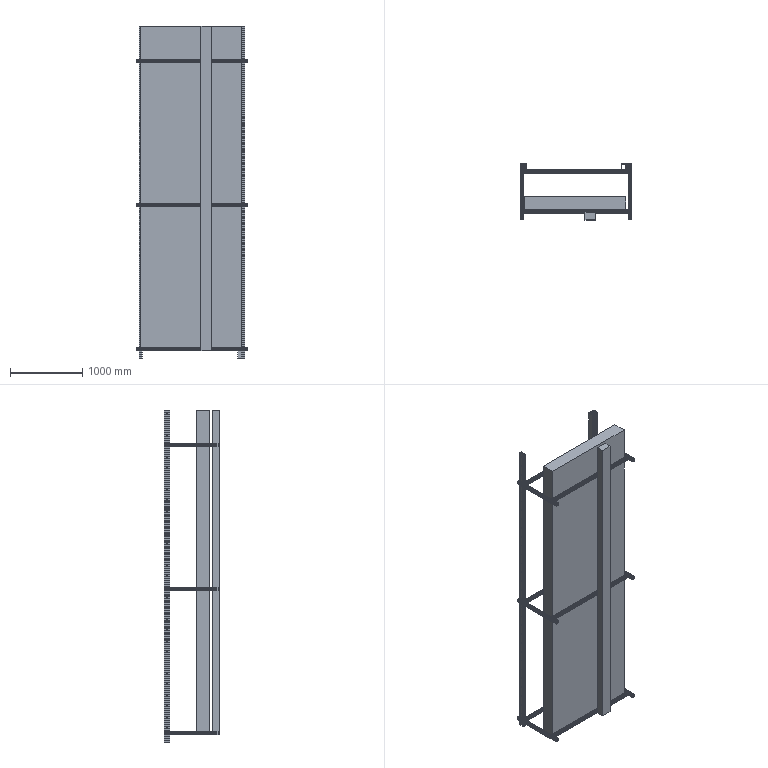Part | SolidWorks | features ICE 4, BossThin 1, Extrusion 1, LPattern 1 | 17 solids | 2118 faces | box 1540 x 775 x 4600 mm | volume 1226148521 mm3 | plane 1342 | cylinder 776 | commonest cylinder face diameters 1 x248 8.2 x248 0.6 x176 10.2 x96 6.8 x8